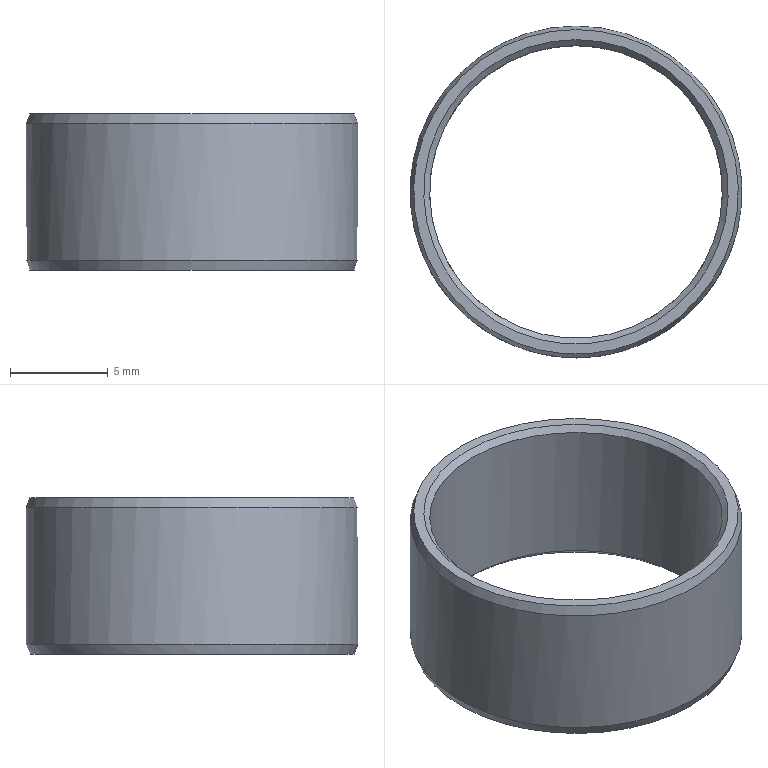Part | NX | features 5003_028_MDZB15-8(Default) 2 | 1 solid | 8 faces | box 17 x 17 x 8 mm | volume 393.001 mm3 | cone 4 | plane 2 | cylinder 2 | commonest cylinder face diameters 15 x1 17 x1
STEP:
#1=CARTESIAN_POINT('',(158.525,-329.8,-237.85));
#2=VERTEX_POINT('',#1);
#3=CARTESIAN_POINT('',(158.525,-322.,-237.85));
#4=DIRECTION('',(0.,0.,1.));
#5=DIRECTION('',(0.,-1.,0.));
#6=AXIS2_PLACEMENT_3D('',#3,#4,#5);
#7=CIRCLE('',#6,7.8);
#8=EDGE_CURVE('',#2,#2,#7,.T.);
#9=ORIENTED_EDGE('',*,*,#8,.T.);
#10=EDGE_LOOP('',(#9));
#11=FACE_BOUND('',#10,.T.);
#12=CARTESIAN_POINT('',(158.525,-330.318,-237.85));
#13=VERTEX_POINT('',#12);
#14=CARTESIAN_POINT('',(158.525,-322.,-237.85));
#15=DIRECTION('',(0.,0.,1.));
#16=DIRECTION('',(0.,-1.,0.));
#17=AXIS2_PLACEMENT_3D('',#14,#15,#16);
#18=CIRCLE('',#17,8.318);
#19=EDGE_CURVE('',#13,#13,#18,.F.);
#20=ORIENTED_EDGE('',*,*,#19,.T.);
#21=EDGE_LOOP('',(#20));
#22=FACE_BOUND('',#21,.T.);
#23=CARTESIAN_POINT('',(166.025,-322.,-237.85));
#24=DIRECTION('',(0.,0.,1.));
#25=DIRECTION('',(0.,-1.,0.));
#26=AXIS2_PLACEMENT_3D('',#23,#24,#25);
#27=PLANE('',#26);
#28=ADVANCED_FACE('',(#11,#22),#27,.F.);
#29=CARTESIAN_POINT('',(158.525,-313.5,-230.35));
#30=VERTEX_POINT('',#29);
#31=CARTESIAN_POINT('',(158.525,-322.,-230.35));
#32=DIRECTION('',(0.,0.,-1.));
#33=DIRECTION('',(0.,1.,0.));
#34=AXIS2_PLACEMENT_3D('',#31,#32,#33);
#35=CIRCLE('',#34,8.5);
#36=EDGE_CURVE('',#30,#30,#35,.T.);
#37=ORIENTED_EDGE('',*,*,#36,.T.);
#38=EDGE_LOOP('',(#37));
#39=FACE_BOUND('',#38,.T.);
#40=CARTESIAN_POINT('',(158.525,-330.5,-237.35));
#41=VERTEX_POINT('',#40);
#42=CARTESIAN_POINT('',(158.525,-322.,-237.35));
#43=DIRECTION('',(0.,0.,1.));
#44=DIRECTION('',(0.,-1.,0.));
#45=AXIS2_PLACEMENT_3D('',#42,#43,#44);
#46=CIRCLE('',#45,8.5);
#47=EDGE_CURVE('',#41,#41,#46,.T.);
#48=ORIENTED_EDGE('',*,*,#47,.T.);
#49=EDGE_LOOP('',(#48));
#50=FACE_BOUND('',#49,.T.);
#51=CARTESIAN_POINT('',(158.525,-322.,-237.85));
#52=DIRECTION('',(0.,0.,-1.));
#53=DIRECTION('',(0.,1.,0.));
#54=AXIS2_PLACEMENT_3D('',#51,#52,#53);
#55=CYLINDRICAL_SURFACE('',#54,8.5);
#56=ADVANCED_FACE('',(#39,#50),#55,.T.);
#57=CARTESIAN_POINT('',(158.525,-314.2,-229.85));
#58=VERTEX_POINT('',#57);
#59=CARTESIAN_POINT('',(158.525,-322.,-229.85));
#60=DIRECTION('',(0.,0.,-1.));
#61=DIRECTION('',(0.,1.,0.));
#62=AXIS2_PLACEMENT_3D('',#59,#60,#61);
#63=CIRCLE('',#62,7.8);
#64=EDGE_CURVE('',#58,#58,#63,.T.);
#65=ORIENTED_EDGE('',*,*,#64,.T.);
#66=EDGE_LOOP('',(#65));
#67=FACE_BOUND('',#66,.T.);
#68=CARTESIAN_POINT('',(158.525,-313.682,-229.85));
#69=VERTEX_POINT('',#68);
#70=CARTESIAN_POINT('',(158.525,-322.,-229.85));
#71=DIRECTION('',(0.,0.,-1.));
#72=DIRECTION('',(0.,1.,0.));
#73=AXIS2_PLACEMENT_3D('',#70,#71,#72);
#74=CIRCLE('',#73,8.318);
#75=EDGE_CURVE('',#69,#69,#74,.F.);
#76=ORIENTED_EDGE('',*,*,#75,.T.);
#77=EDGE_LOOP('',(#76));
#78=FACE_BOUND('',#77,.T.);
#79=CARTESIAN_POINT('',(166.025,-322.,-229.85));
#80=DIRECTION('',(0.,0.,-1.));
#81=DIRECTION('',(0.,1.,0.));
#82=AXIS2_PLACEMENT_3D('',#79,#80,#81);
#83=PLANE('',#82);
#84=ADVANCED_FACE('',(#67,#78),#83,.F.);
#85=CARTESIAN_POINT('',(158.525,-329.5,-237.55));
#86=VERTEX_POINT('',#85);
#87=CARTESIAN_POINT('',(158.525,-322.,-237.55));
#88=DIRECTION('',(0.,0.,1.));
#89=DIRECTION('',(0.,-1.,0.));
#90=AXIS2_PLACEMENT_3D('',#87,#88,#89);
#91=CIRCLE('',#90,7.5);
#92=EDGE_CURVE('',#86,#86,#91,.F.);
#93=ORIENTED_EDGE('',*,*,#92,.T.);
#94=EDGE_LOOP('',(#93));
#95=FACE_BOUND('',#94,.T.);
#96=CARTESIAN_POINT('',(158.525,-314.5,-230.15));
#97=VERTEX_POINT('',#96);
#98=CARTESIAN_POINT('',(158.525,-322.,-230.15));
#99=DIRECTION('',(0.,0.,-1.));
#100=DIRECTION('',(0.,1.,0.));
#101=AXIS2_PLACEMENT_3D('',#98,#99,#100);
#102=CIRCLE('',#101,7.5);
#103=EDGE_CURVE('',#97,#97,#102,.F.);
#104=ORIENTED_EDGE('',*,*,#103,.T.);
#105=EDGE_LOOP('',(#104));
#106=FACE_BOUND('',#105,.T.);
#107=CARTESIAN_POINT('',(158.525,-322.,-237.85));
#108=DIRECTION('',(0.,0.,-1.));
#109=DIRECTION('',(0.,1.,0.));
#110=AXIS2_PLACEMENT_3D('',#107,#108,#109);
#111=CYLINDRICAL_SURFACE('',#110,7.5);
#112=ADVANCED_FACE('',(#95,#106),#111,.F.);
#113=ORIENTED_EDGE('',*,*,#75,.F.);
#114=EDGE_LOOP('',(#113));
#115=FACE_BOUND('',#114,.T.);
#116=ORIENTED_EDGE('',*,*,#36,.F.);
#117=EDGE_LOOP('',(#116));
#118=FACE_BOUND('',#117,.T.);
#119=CARTESIAN_POINT('',(158.525,-322.,-230.35));
#120=DIRECTION('',(0.,0.,-1.));
#121=DIRECTION('',(0.,1.,0.));
#122=AXIS2_PLACEMENT_3D('',#119,#120,#121);
#123=CONICAL_SURFACE('',#122,8.5,0.3491);
#124=ADVANCED_FACE('',(#115,#118),#123,.T.);
#125=ORIENTED_EDGE('',*,*,#47,.F.);
#126=EDGE_LOOP('',(#125));
#127=FACE_BOUND('',#126,.T.);
#128=ORIENTED_EDGE('',*,*,#19,.F.);
#129=EDGE_LOOP('',(#128));
#130=FACE_BOUND('',#129,.T.);
#131=CARTESIAN_POINT('',(158.525,-322.,-237.85));
#132=DIRECTION('',(0.,0.,1.));
#133=DIRECTION('',(0.,-1.,0.));
#134=AXIS2_PLACEMENT_3D('',#131,#132,#133);
#135=CONICAL_SURFACE('',#134,8.318,0.3491);
#136=ADVANCED_FACE('',(#127,#130),#135,.T.);
#137=ORIENTED_EDGE('',*,*,#8,.F.);
#138=EDGE_LOOP('',(#137));
#139=FACE_BOUND('',#138,.T.);
#140=ORIENTED_EDGE('',*,*,#92,.F.);
#141=EDGE_LOOP('',(#140));
#142=FACE_BOUND('',#141,.T.);
#143=CARTESIAN_POINT('',(158.525,-322.,-237.55));
#144=DIRECTION('',(0.,0.,-1.));
#145=DIRECTION('',(0.,1.,0.));
#146=AXIS2_PLACEMENT_3D('',#143,#144,#145);
#147=CONICAL_SURFACE('',#146,7.5,0.7854);
#148=ADVANCED_FACE('',(#139,#142),#147,.F.);
#149=ORIENTED_EDGE('',*,*,#103,.F.);
#150=EDGE_LOOP('',(#149));
#151=FACE_BOUND('',#150,.T.);
#152=ORIENTED_EDGE('',*,*,#64,.F.);
#153=EDGE_LOOP('',(#152));
#154=FACE_BOUND('',#153,.T.);
#155=CARTESIAN_POINT('',(158.525,-322.,-229.85));
#156=DIRECTION('',(0.,0.,1.));
#157=DIRECTION('',(0.,-1.,0.));
#158=AXIS2_PLACEMENT_3D('',#155,#156,#157);
#159=CONICAL_SURFACE('',#158,7.8,0.7854);
#160=ADVANCED_FACE('',(#151,#154),#159,.F.);
#161=CLOSED_SHELL('',(#28,#56,#84,#112,#124,#136,#148,#160));
#162=MANIFOLD_SOLID_BREP('',#161);
#163=(LENGTH_UNIT()NAMED_UNIT(*)SI_UNIT(.MILLI.,.METRE.));
#164=UNCERTAINTY_MEASURE_WITH_UNIT(LENGTH_MEASURE(0.00001),#163,'','');
#165=(NAMED_UNIT(*)PLANE_ANGLE_UNIT()SI_UNIT($,.RADIAN.));
#166=(NAMED_UNIT(*)SI_UNIT($,.STERADIAN.)SOLID_ANGLE_UNIT());
#167=(GEOMETRIC_REPRESENTATION_CONTEXT(3)GLOBAL_UNCERTAINTY_ASSIGNED_CONTEXT((#164))GLOBAL_UNIT_ASSIGNED_CONTEXT((#163,#165,#166))REPRESENTATION_CONTEXT('',''));
#168=ADVANCED_BREP_SHAPE_REPRESENTATION('',(#162),#167);